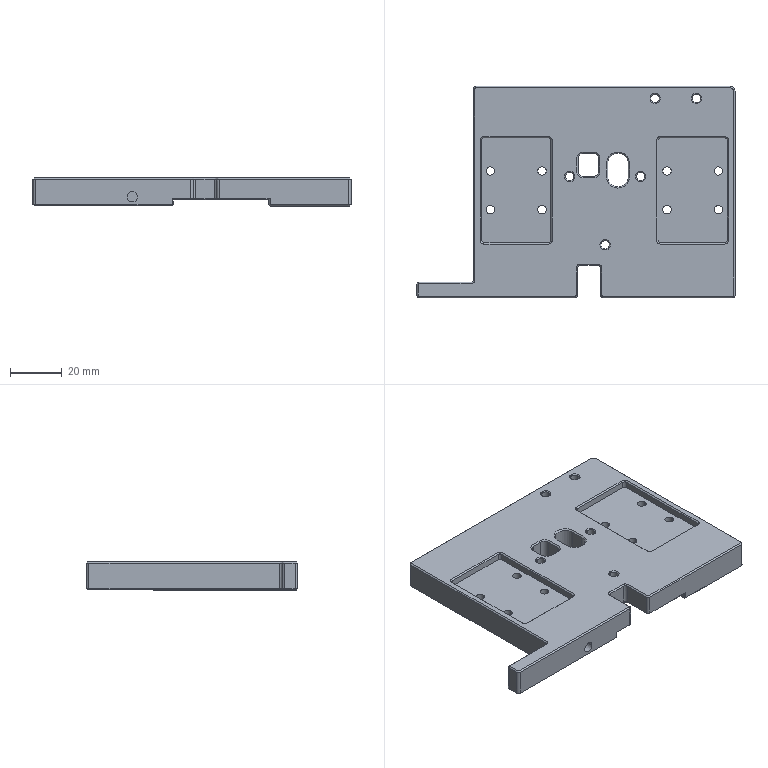Part | 1 solid | 282 faces | box 123.41 x 82 x 11.078 mm | volume 71402 mm3 | plane 142 | cylinder 72 | cone 65 | spline 3 | commonest cylinder face diameters 3.3 x26 2 x19 6.5 x16 4 x8 8 x3